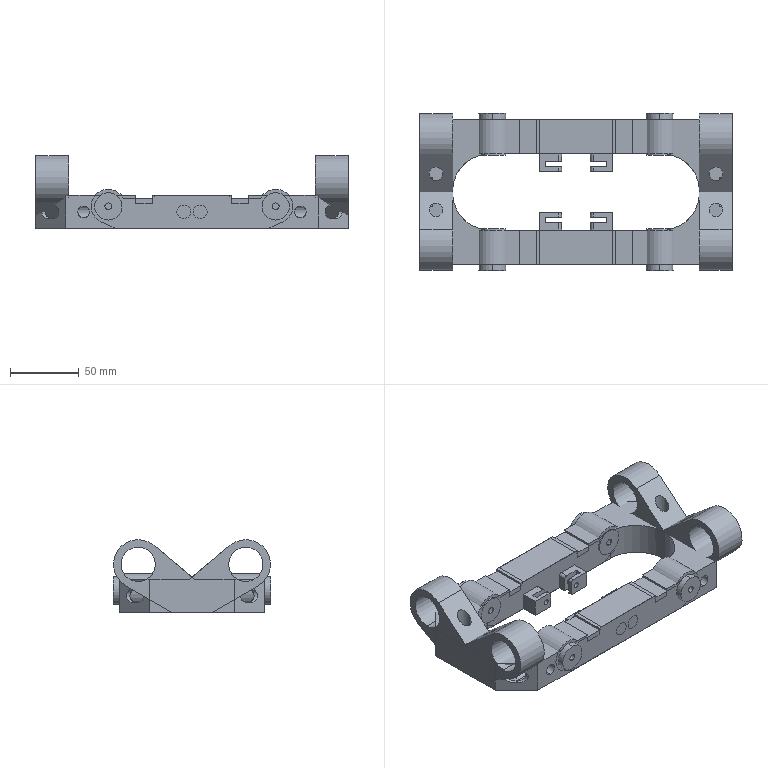NC program | Mastercam | posted with a generic post | part box 228 x 114.503 x 53 mm
Whole program:
%
:0001()
(MATERIAL - ALUMINUM MM - 2024)
(T1|2.5 DR |H1)
(T2|4.2 DR |H2)
(T3|50 FEM |H3)
N100 G21
N102 G0 G17 G40 G80 G90 G94 G98
N104 G0 G28 G91 Z0.
N106 G0 G28 X0. Y0.
(2.5 DR |TOOL - 1|DIA. OFF. - 1|LEN. - 1|TOOL DIA. - 2.5)
N108 T1 M6
N110 G0 G54 G90 X-129.548 Y5.75 C0. B0. S1200 M3
N112 G43 H1 Z62.5
N114 G83 G98 Z20.5 R39.5 Q1. F70.
N116 G80
N118 M5
N120 G0 G28 G91 Z0.
N122 G28
N124 M01
N126 G0 G17 G40 G80 G90 G94 G98
N128 G0 G28 G91 Z0.
(4.2 DR |TOOL - 2|DIA. OFF. - 2|LEN. - 2|TOOL DIA. - 4.2)
N130 T2 M6
N132 G0 G54 G90 X-129.548 Y5.75 C0. B0. S1000 M3
N134 G43 H2 Z62.5
N136 G83 G98 Z31.5 R39.5 Q1.5 F100.
N138 G80
N140 M5
N142 G0 G28 G91 Z0.
N144 G28
N146 M01
N148 G0 G17 G40 G80 G90 G94 G98
N150 G0 G28 G91 Z0.
(50 FEM |TOOL - 3|DIA. OFF. - 3|LEN. - 3|TOOL DIA. - 50.)
N152 T3 M6
N154 G0 G54 G90 X-111.548 Y44.5 C0. B0. S1400 M3
N156 G43 H3 Z80.5
N158 Z35.5
N160 G1 Z30.5 F600.
N162 Y12. F200.
N164 Y-.5
N166 Y-33.
N168 G0 Z80.5
N170 M5
N172 G0 G28 G91 Z0.
N174 G28
N176 M01
N178 G0 G17 G40 G80 G90 G94 G98
N180 G0 G28 G91 Z0.
(2.5 DR |TOOL - 1|DIA. OFF. - 1|LEN. - 1|TOOL DIA. - 2.5)
N182 T1 M6
N184 G0 G54 G90 X-129.548 Y-5.75 C0. B0. S1200 M3
N186 G43 H1 Z62.5
N188 G83 G98 Z20.5 R39.5 Q1. F70.
N190 G80
N192 M5
N194 G0 G28 G91 Z0.
N196 G28
N198 M01
N200 G0 G17 G40 G80 G90 G94 G98
N202 G0 G28 G91 Z0.
(4.2 DR |TOOL - 2|DIA. OFF. - 2|LEN. - 2|TOOL DIA. - 4.2)
N204 T2 M6
N206 G0 G54 G90 X-129.548 Y-5.75 C0. B0. S1000 M3
N208 G43 H2 Z62.5
N210 G83 G98 Z31.5 R39.5 Q1.5 F100.
N212 G80
N214 M5
N216 G0 G28 G91 Z0.
N218 G28
N220 M01
N222 G0 G17 G40 G80 G90 G94 G98
N224 G0 G28 G91 Z0.
(50 FEM |TOOL - 3|DIA. OFF. - 3|LEN. - 3|TOOL DIA. - 50.)
N226 T3 M6
N228 G0 G54 G90 X-111.548 Y33. C0. B0. S1400 M3
N230 G43 H3 Z80.5
N232 Z35.5
N234 G1 Z30.5 F600.
N236 Y.5 F50.
N238 Y-12.
N240 Y-44.5
N242 G0 Z80.5
N244 M5
N246 G0 G28 G91 Z0.
N248 G0 G28 X0. Y0.
N250 G28
N252 M30
%